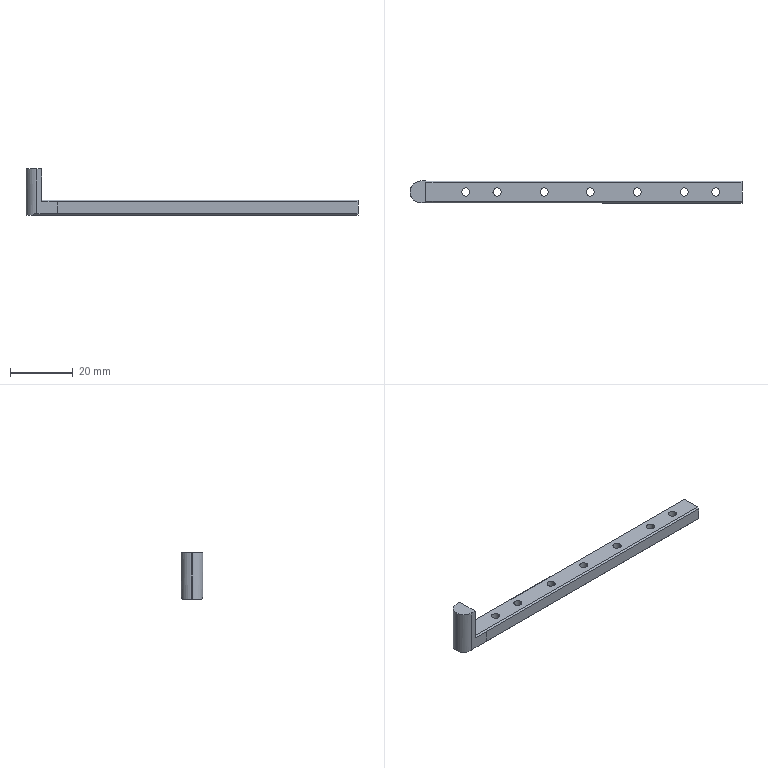Part | SolidWorks | features Chamfer 1, Extrusion 1, Fillet 1, ICE 1 | 1 solid | 34 faces | box 105.759 x 6.991 x 14.8 mm | volume 3589 mm3 | plane 18 | cylinder 16 | commonest cylinder face diameters 2.6 x14 6.98 x2
STEP:
#1=CARTESIAN_POINT('',(-94.656,-26.837,4.8));
#2=VERTEX_POINT('',#1);
#3=CARTESIAN_POINT('',(-92.056,-26.837,4.8));
#4=VERTEX_POINT('',#3);
#5=CARTESIAN_POINT('',(-93.356,-26.837,4.8));
#6=DIRECTION('',(0.,0.,1.));
#7=DIRECTION('',(1.,0.,0.));
#8=AXIS2_PLACEMENT_3D('',#5,#6,#7);
#9=CIRCLE('',#8,1.3);
#10=EDGE_CURVE('',#2,#4,#9,.T.);
#11=ORIENTED_EDGE('',*,*,#10,.T.);
#12=CARTESIAN_POINT('',(-92.056,-26.837,0.));
#13=VERTEX_POINT('',#12);
#14=CARTESIAN_POINT('',(-92.056,-26.837,4.8));
#15=DIRECTION('',(0.,0.,-1.));
#16=VECTOR('',#15,1000.);
#17=LINE('',#14,#16);
#18=EDGE_CURVE('',#4,#13,#17,.T.);
#19=ORIENTED_EDGE('',*,*,#18,.T.);
#20=CARTESIAN_POINT('',(-94.656,-26.837,0.));
#21=VERTEX_POINT('',#20);
#22=CARTESIAN_POINT('',(-93.356,-26.837,0.));
#23=DIRECTION('',(0.,0.,1.));
#24=DIRECTION('',(1.,0.,0.));
#25=AXIS2_PLACEMENT_3D('',#22,#23,#24);
#26=CIRCLE('',#25,1.3);
#27=EDGE_CURVE('',#21,#13,#26,.T.);
#28=ORIENTED_EDGE('',*,*,#27,.F.);
#29=CARTESIAN_POINT('',(-94.656,-26.837,4.8));
#30=DIRECTION('',(0.,0.,-1.));
#31=VECTOR('',#30,1000.);
#32=LINE('',#29,#31);
#33=EDGE_CURVE('',#2,#21,#32,.T.);
#34=ORIENTED_EDGE('',*,*,#33,.F.);
#35=EDGE_LOOP('',(#11,#19,#28,#34));
#36=FACE_OUTER_BOUND('',#35,.T.);
#37=CARTESIAN_POINT('',(-93.356,-26.837,4.8));
#38=DIRECTION('',(0.,0.,-1.));
#39=DIRECTION('',(-1.,0.,0.));
#40=AXIS2_PLACEMENT_3D('',#37,#38,#39);
#41=CYLINDRICAL_SURFACE('',#40,1.3);
#42=ADVANCED_FACE('',(#36),#41,.F.);
#43=CARTESIAN_POINT('',(-104.656,-26.837,4.8));
#44=VERTEX_POINT('',#43);
#45=CARTESIAN_POINT('',(-102.056,-26.837,4.8));
#46=VERTEX_POINT('',#45);
#47=CARTESIAN_POINT('',(-103.356,-26.837,4.8));
#48=DIRECTION('',(0.,0.,1.));
#49=DIRECTION('',(1.,0.,0.));
#50=AXIS2_PLACEMENT_3D('',#47,#48,#49);
#51=CIRCLE('',#50,1.3);
#52=EDGE_CURVE('',#44,#46,#51,.T.);
#53=ORIENTED_EDGE('',*,*,#52,.T.);
#54=CARTESIAN_POINT('',(-102.056,-26.837,0.));
#55=VERTEX_POINT('',#54);
#56=CARTESIAN_POINT('',(-102.056,-26.837,4.8));
#57=DIRECTION('',(0.,0.,-1.));
#58=VECTOR('',#57,1000.);
#59=LINE('',#56,#58);
#60=EDGE_CURVE('',#46,#55,#59,.T.);
#61=ORIENTED_EDGE('',*,*,#60,.T.);
#62=CARTESIAN_POINT('',(-104.656,-26.837,0.));
#63=VERTEX_POINT('',#62);
#64=CARTESIAN_POINT('',(-103.356,-26.837,0.));
#65=DIRECTION('',(0.,0.,1.));
#66=DIRECTION('',(1.,0.,0.));
#67=AXIS2_PLACEMENT_3D('',#64,#65,#66);
#68=CIRCLE('',#67,1.3);
#69=EDGE_CURVE('',#63,#55,#68,.T.);
#70=ORIENTED_EDGE('',*,*,#69,.F.);
#71=CARTESIAN_POINT('',(-104.656,-26.837,4.8));
#72=DIRECTION('',(0.,0.,-1.));
#73=VECTOR('',#72,1000.);
#74=LINE('',#71,#73);
#75=EDGE_CURVE('',#44,#63,#74,.T.);
#76=ORIENTED_EDGE('',*,*,#75,.F.);
#77=EDGE_LOOP('',(#53,#61,#70,#76));
#78=FACE_OUTER_BOUND('',#77,.T.);
#79=CARTESIAN_POINT('',(-103.356,-26.837,4.8));
#80=DIRECTION('',(0.,0.,-1.));
#81=DIRECTION('',(-1.,0.,0.));
#82=AXIS2_PLACEMENT_3D('',#79,#80,#81);
#83=CYLINDRICAL_SURFACE('',#82,1.3);
#84=ADVANCED_FACE('',(#78),#83,.F.);
#85=CARTESIAN_POINT('',(-119.656,-26.837,4.8));
#86=VERTEX_POINT('',#85);
#87=CARTESIAN_POINT('',(-117.056,-26.837,4.8));
#88=VERTEX_POINT('',#87);
#89=CARTESIAN_POINT('',(-118.356,-26.837,4.8));
#90=DIRECTION('',(0.,0.,1.));
#91=DIRECTION('',(1.,0.,0.));
#92=AXIS2_PLACEMENT_3D('',#89,#90,#91);
#93=CIRCLE('',#92,1.3);
#94=EDGE_CURVE('',#86,#88,#93,.T.);
#95=ORIENTED_EDGE('',*,*,#94,.T.);
#96=CARTESIAN_POINT('',(-117.056,-26.837,0.));
#97=VERTEX_POINT('',#96);
#98=CARTESIAN_POINT('',(-117.056,-26.837,4.8));
#99=DIRECTION('',(0.,0.,-1.));
#100=VECTOR('',#99,1000.);
#101=LINE('',#98,#100);
#102=EDGE_CURVE('',#88,#97,#101,.T.);
#103=ORIENTED_EDGE('',*,*,#102,.T.);
#104=CARTESIAN_POINT('',(-119.656,-26.837,0.));
#105=VERTEX_POINT('',#104);
#106=CARTESIAN_POINT('',(-118.356,-26.837,0.));
#107=DIRECTION('',(0.,0.,1.));
#108=DIRECTION('',(1.,0.,0.));
#109=AXIS2_PLACEMENT_3D('',#106,#107,#108);
#110=CIRCLE('',#109,1.3);
#111=EDGE_CURVE('',#105,#97,#110,.T.);
#112=ORIENTED_EDGE('',*,*,#111,.F.);
#113=CARTESIAN_POINT('',(-119.656,-26.837,4.8));
#114=DIRECTION('',(0.,0.,-1.));
#115=VECTOR('',#114,1000.);
#116=LINE('',#113,#115);
#117=EDGE_CURVE('',#86,#105,#116,.T.);
#118=ORIENTED_EDGE('',*,*,#117,.F.);
#119=EDGE_LOOP('',(#95,#103,#112,#118));
#120=FACE_OUTER_BOUND('',#119,.T.);
#121=CARTESIAN_POINT('',(-118.356,-26.837,4.8));
#122=DIRECTION('',(0.,0.,-1.));
#123=DIRECTION('',(-1.,0.,0.));
#124=AXIS2_PLACEMENT_3D('',#121,#122,#123);
#125=CYLINDRICAL_SURFACE('',#124,1.3);
#126=ADVANCED_FACE('',(#120),#125,.F.);
#127=CARTESIAN_POINT('',(-164.311,-26.837,4.8));
#128=VERTEX_POINT('',#127);
#129=CARTESIAN_POINT('',(-161.711,-26.837,4.8));
#130=VERTEX_POINT('',#129);
#131=CARTESIAN_POINT('',(-163.011,-26.837,4.8));
#132=DIRECTION('',(0.,0.,1.));
#133=DIRECTION('',(1.,0.,0.));
#134=AXIS2_PLACEMENT_3D('',#131,#132,#133);
#135=CIRCLE('',#134,1.3);
#136=EDGE_CURVE('',#128,#130,#135,.T.);
#137=ORIENTED_EDGE('',*,*,#136,.T.);
#138=CARTESIAN_POINT('',(-161.711,-26.837,0.));
#139=VERTEX_POINT('',#138);
#140=CARTESIAN_POINT('',(-161.711,-26.837,4.8));
#141=DIRECTION('',(0.,0.,-1.));
#142=VECTOR('',#141,1000.);
#143=LINE('',#140,#142);
#144=EDGE_CURVE('',#130,#139,#143,.T.);
#145=ORIENTED_EDGE('',*,*,#144,.T.);
#146=CARTESIAN_POINT('',(-164.311,-26.837,0.));
#147=VERTEX_POINT('',#146);
#148=CARTESIAN_POINT('',(-163.011,-26.837,0.));
#149=DIRECTION('',(0.,0.,1.));
#150=DIRECTION('',(1.,0.,0.));
#151=AXIS2_PLACEMENT_3D('',#148,#149,#150);
#152=CIRCLE('',#151,1.3);
#153=EDGE_CURVE('',#147,#139,#152,.T.);
#154=ORIENTED_EDGE('',*,*,#153,.F.);
#155=CARTESIAN_POINT('',(-164.311,-26.837,4.8));
#156=DIRECTION('',(0.,0.,-1.));
#157=VECTOR('',#156,1000.);
#158=LINE('',#155,#157);
#159=EDGE_CURVE('',#128,#147,#158,.T.);
#160=ORIENTED_EDGE('',*,*,#159,.F.);
#161=EDGE_LOOP('',(#137,#145,#154,#160));
#162=FACE_OUTER_BOUND('',#161,.T.);
#163=CARTESIAN_POINT('',(-163.011,-26.837,4.8));
#164=DIRECTION('',(0.,0.,-1.));
#165=DIRECTION('',(-1.,0.,0.));
#166=AXIS2_PLACEMENT_3D('',#163,#164,#165);
#167=CYLINDRICAL_SURFACE('',#166,1.3);
#168=ADVANCED_FACE('',(#162),#167,.F.);
#169=CARTESIAN_POINT('',(-149.311,-26.837,4.8));
#170=VERTEX_POINT('',#169);
#171=CARTESIAN_POINT('',(-146.711,-26.837,4.8));
#172=VERTEX_POINT('',#171);
#173=CARTESIAN_POINT('',(-148.011,-26.837,4.8));
#174=DIRECTION('',(0.,0.,1.));
#175=DIRECTION('',(1.,0.,0.));
#176=AXIS2_PLACEMENT_3D('',#173,#174,#175);
#177=CIRCLE('',#176,1.3);
#178=EDGE_CURVE('',#170,#172,#177,.T.);
#179=ORIENTED_EDGE('',*,*,#178,.T.);
#180=CARTESIAN_POINT('',(-146.711,-26.837,0.));
#181=VERTEX_POINT('',#180);
#182=CARTESIAN_POINT('',(-146.711,-26.837,4.8));
#183=DIRECTION('',(0.,0.,-1.));
#184=VECTOR('',#183,1000.);
#185=LINE('',#182,#184);
#186=EDGE_CURVE('',#172,#181,#185,.T.);
#187=ORIENTED_EDGE('',*,*,#186,.T.);
#188=CARTESIAN_POINT('',(-149.311,-26.837,0.));
#189=VERTEX_POINT('',#188);
#190=CARTESIAN_POINT('',(-148.011,-26.837,0.));
#191=DIRECTION('',(0.,0.,1.));
#192=DIRECTION('',(1.,0.,0.));
#193=AXIS2_PLACEMENT_3D('',#190,#191,#192);
#194=CIRCLE('',#193,1.3);
#195=EDGE_CURVE('',#189,#181,#194,.T.);
#196=ORIENTED_EDGE('',*,*,#195,.F.);
#197=CARTESIAN_POINT('',(-149.311,-26.837,4.8));
#198=DIRECTION('',(0.,0.,-1.));
#199=VECTOR('',#198,1000.);
#200=LINE('',#197,#199);
#201=EDGE_CURVE('',#170,#189,#200,.T.);
#202=ORIENTED_EDGE('',*,*,#201,.F.);
#203=EDGE_LOOP('',(#179,#187,#196,#202));
#204=FACE_OUTER_BOUND('',#203,.T.);
#205=CARTESIAN_POINT('',(-148.011,-26.837,4.8));
#206=DIRECTION('',(0.,0.,-1.));
#207=DIRECTION('',(-1.,0.,0.));
#208=AXIS2_PLACEMENT_3D('',#205,#206,#207);
#209=CYLINDRICAL_SURFACE('',#208,1.3);
#210=ADVANCED_FACE('',(#204),#209,.F.);
#211=CARTESIAN_POINT('',(-134.656,-26.837,4.8));
#212=VERTEX_POINT('',#211);
#213=CARTESIAN_POINT('',(-132.056,-26.837,4.8));
#214=VERTEX_POINT('',#213);
#215=CARTESIAN_POINT('',(-133.356,-26.837,4.8));
#216=DIRECTION('',(0.,0.,1.));
#217=DIRECTION('',(1.,0.,0.));
#218=AXIS2_PLACEMENT_3D('',#215,#216,#217);
#219=CIRCLE('',#218,1.3);
#220=EDGE_CURVE('',#212,#214,#219,.T.);
#221=ORIENTED_EDGE('',*,*,#220,.T.);
#222=CARTESIAN_POINT('',(-132.056,-26.837,0.));
#223=VERTEX_POINT('',#222);
#224=CARTESIAN_POINT('',(-132.056,-26.837,4.8));
#225=DIRECTION('',(0.,0.,-1.));
#226=VECTOR('',#225,1000.);
#227=LINE('',#224,#226);
#228=EDGE_CURVE('',#214,#223,#227,.T.);
#229=ORIENTED_EDGE('',*,*,#228,.T.);
#230=CARTESIAN_POINT('',(-134.656,-26.837,0.));
#231=VERTEX_POINT('',#230);
#232=CARTESIAN_POINT('',(-133.356,-26.837,0.));
#233=DIRECTION('',(0.,0.,1.));
#234=DIRECTION('',(1.,0.,0.));
#235=AXIS2_PLACEMENT_3D('',#232,#233,#234);
#236=CIRCLE('',#235,1.3);
#237=EDGE_CURVE('',#231,#223,#236,.T.);
#238=ORIENTED_EDGE('',*,*,#237,.F.);
#239=CARTESIAN_POINT('',(-134.656,-26.837,4.8));
#240=DIRECTION('',(0.,0.,-1.));
#241=VECTOR('',#240,1000.);
#242=LINE('',#239,#241);
#243=EDGE_CURVE('',#212,#231,#242,.T.);
#244=ORIENTED_EDGE('',*,*,#243,.F.);
#245=EDGE_LOOP('',(#221,#229,#238,#244));
#246=FACE_OUTER_BOUND('',#245,.T.);
#247=CARTESIAN_POINT('',(-133.356,-26.837,4.8));
#248=DIRECTION('',(0.,0.,-1.));
#249=DIRECTION('',(-1.,0.,0.));
#250=AXIS2_PLACEMENT_3D('',#247,#248,#249);
#251=CYLINDRICAL_SURFACE('',#250,1.3);
#252=ADVANCED_FACE('',(#246),#251,.F.);
#253=CARTESIAN_POINT('',(-174.311,-26.837,4.8));
#254=VERTEX_POINT('',#253);
#255=CARTESIAN_POINT('',(-171.711,-26.837,4.8));
#256=VERTEX_POINT('',#255);
#257=CARTESIAN_POINT('',(-173.011,-26.837,4.8));
#258=DIRECTION('',(0.,0.,1.));
#259=DIRECTION('',(1.,0.,0.));
#260=AXIS2_PLACEMENT_3D('',#257,#258,#259);
#261=CIRCLE('',#260,1.3);
#262=EDGE_CURVE('',#254,#256,#261,.T.);
#263=ORIENTED_EDGE('',*,*,#262,.T.);
#264=CARTESIAN_POINT('',(-171.711,-26.837,0.));
#265=VERTEX_POINT('',#264);
#266=CARTESIAN_POINT('',(-171.711,-26.837,4.8));
#267=DIRECTION('',(0.,0.,-1.));
#268=VECTOR('',#267,1000.);
#269=LINE('',#266,#268);
#270=EDGE_CURVE('',#256,#265,#269,.T.);
#271=ORIENTED_EDGE('',*,*,#270,.T.);
#272=CARTESIAN_POINT('',(-174.311,-26.837,0.));
#273=VERTEX_POINT('',#272);
#274=CARTESIAN_POINT('',(-173.011,-26.837,0.));
#275=DIRECTION('',(0.,0.,1.));
#276=DIRECTION('',(1.,0.,0.));
#277=AXIS2_PLACEMENT_3D('',#274,#275,#276);
#278=CIRCLE('',#277,1.3);
#279=EDGE_CURVE('',#273,#265,#278,.T.);
#280=ORIENTED_EDGE('',*,*,#279,.F.);
#281=CARTESIAN_POINT('',(-174.311,-26.837,4.8));
#282=DIRECTION('',(0.,0.,-1.));
#283=VECTOR('',#282,1000.);
#284=LINE('',#281,#283);
#285=EDGE_CURVE('',#254,#273,#284,.T.);
#286=ORIENTED_EDGE('',*,*,#285,.F.);
#287=EDGE_LOOP('',(#263,#271,#280,#286));
#288=FACE_OUTER_BOUND('',#287,.T.);
#289=CARTESIAN_POINT('',(-173.011,-26.837,4.8));
#290=DIRECTION('',(0.,0.,-1.));
#291=DIRECTION('',(-1.,0.,0.));
#292=AXIS2_PLACEMENT_3D('',#289,#290,#291);
#293=CYLINDRICAL_SURFACE('',#292,1.3);
#294=ADVANCED_FACE('',(#288),#293,.F.);
#295=ORIENTED_EDGE('',*,*,#10,.F.);
#296=CARTESIAN_POINT('',(-93.356,-26.837,4.8));
#297=DIRECTION('',(0.,0.,1.));
#298=DIRECTION('',(1.,0.,0.));
#299=AXIS2_PLACEMENT_3D('',#296,#297,#298);
#300=CIRCLE('',#299,1.3);
#301=EDGE_CURVE('',#4,#2,#300,.T.);
#302=ORIENTED_EDGE('',*,*,#301,.F.);
#303=EDGE_LOOP('',(#295,#302));
#304=FACE_BOUND('',#303,.T.);
#305=ORIENTED_EDGE('',*,*,#52,.F.);
#306=CARTESIAN_POINT('',(-103.356,-26.837,4.8));
#307=DIRECTION('',(0.,0.,1.));
#308=DIRECTION('',(1.,0.,0.));
#309=AXIS2_PLACEMENT_3D('',#306,#307,#308);
#310=CIRCLE('',#309,1.3);
#311=EDGE_CURVE('',#46,#44,#310,.T.);
#312=ORIENTED_EDGE('',*,*,#311,.F.);
#313=EDGE_LOOP('',(#305,#312));
#314=FACE_BOUND('',#313,.T.);
#315=ORIENTED_EDGE('',*,*,#94,.F.);
#316=CARTESIAN_POINT('',(-118.356,-26.837,4.8));
#317=DIRECTION('',(0.,0.,1.));
#318=DIRECTION('',(1.,0.,0.));
#319=AXIS2_PLACEMENT_3D('',#316,#317,#318);
#320=CIRCLE('',#319,1.3);
#321=EDGE_CURVE('',#88,#86,#320,.T.);
#322=ORIENTED_EDGE('',*,*,#321,.F.);
#323=EDGE_LOOP('',(#315,#322));
#324=FACE_BOUND('',#323,.T.);
#325=ORIENTED_EDGE('',*,*,#136,.F.);
#326=CARTESIAN_POINT('',(-163.011,-26.837,4.8));
#327=DIRECTION('',(0.,0.,1.));
#328=DIRECTION('',(1.,0.,0.));
#329=AXIS2_PLACEMENT_3D('',#326,#327,#328);
#330=CIRCLE('',#329,1.3);
#331=EDGE_CURVE('',#130,#128,#330,.T.);
#332=ORIENTED_EDGE('',*,*,#331,.F.);
#333=EDGE_LOOP('',(#325,#332));
#334=FACE_BOUND('',#333,.T.);
#335=ORIENTED_EDGE('',*,*,#178,.F.);
#336=CARTESIAN_POINT('',(-148.011,-26.837,4.8));
#337=DIRECTION('',(0.,0.,1.));
#338=DIRECTION('',(1.,0.,0.));
#339=AXIS2_PLACEMENT_3D('',#336,#337,#338);
#340=CIRCLE('',#339,1.3);
#341=EDGE_CURVE('',#172,#170,#340,.T.);
#342=ORIENTED_EDGE('',*,*,#341,.F.);
#343=EDGE_LOOP('',(#335,#342));
#344=FACE_BOUND('',#343,.T.);
#345=ORIENTED_EDGE('',*,*,#220,.F.);
#346=CARTESIAN_POINT('',(-133.356,-26.837,4.8));
#347=DIRECTION('',(0.,0.,1.));
#348=DIRECTION('',(1.,0.,0.));
#349=AXIS2_PLACEMENT_3D('',#346,#347,#348);
#350=CIRCLE('',#349,1.3);
#351=EDGE_CURVE('',#214,#212,#350,.T.);
#352=ORIENTED_EDGE('',*,*,#351,.F.);
#353=EDGE_LOOP('',(#345,#352));
#354=FACE_BOUND('',#353,.T.);
#355=ORIENTED_EDGE('',*,*,#262,.F.);
#356=CARTESIAN_POINT('',(-173.011,-26.837,4.8));
#357=DIRECTION('',(0.,0.,1.));
#358=DIRECTION('',(1.,0.,0.));
#359=AXIS2_PLACEMENT_3D('',#356,#357,#358);
#360=CIRCLE('',#359,1.3);
#361=EDGE_CURVE('',#256,#254,#360,.T.);
#362=ORIENTED_EDGE('',*,*,#361,.F.);
#363=EDGE_LOOP('',(#355,#362));
#364=FACE_BOUND('',#363,.T.);
#365=CARTESIAN_POINT('',(-185.746,-29.829,4.8));
#366=VERTEX_POINT('',#365);
#367=CARTESIAN_POINT('',(-185.746,-23.846,4.8));
#368=VERTEX_POINT('',#367);
#369=CARTESIAN_POINT('',(-185.746,-23.346,4.8));
#370=DIRECTION('',(0.,1.,0.));
#371=VECTOR('',#370,1000.);
#372=LINE('',#369,#371);
#373=EDGE_CURVE('',#366,#368,#372,.T.);
#374=ORIENTED_EDGE('',*,*,#373,.F.);
#375=CARTESIAN_POINT('',(-180.746,-29.829,4.8));
#376=VERTEX_POINT('',#375);
#377=CARTESIAN_POINT('',(0.,-29.829,4.8));
#378=DIRECTION('',(1.,0.,0.));
#379=VECTOR('',#378,1000.);
#380=LINE('',#377,#379);
#381=EDGE_CURVE('',#366,#376,#380,.T.);
#382=ORIENTED_EDGE('',*,*,#381,.T.);
#383=CARTESIAN_POINT('',(-84.986,-29.833,4.8));
#384=VERTEX_POINT('',#383);
#385=CARTESIAN_POINT('',(-0.001305,-29.836,4.8));
#386=DIRECTION('',(1.,-0.00004375,0.));
#387=VECTOR('',#386,1000.);
#388=LINE('',#385,#387);
#389=EDGE_CURVE('',#376,#384,#388,.T.);
#390=ORIENTED_EDGE('',*,*,#389,.T.);
#391=CARTESIAN_POINT('',(-84.986,-23.841,4.8));
#392=VERTEX_POINT('',#391);
#393=CARTESIAN_POINT('',(-84.986,-23.341,4.8));
#394=DIRECTION('',(0.,1.,0.));
#395=VECTOR('',#394,1000.);
#396=LINE('',#393,#395);
#397=EDGE_CURVE('',#384,#392,#396,.T.);
#398=ORIENTED_EDGE('',*,*,#397,.T.);
#399=CARTESIAN_POINT('',(-180.746,-23.846,4.8));
#400=VERTEX_POINT('',#399);
#401=CARTESIAN_POINT('',(0.001044,-23.838,4.8));
#402=DIRECTION('',(-1.,-0.00004379,0.));
#403=VECTOR('',#402,1000.);
#404=LINE('',#401,#403);
#405=EDGE_CURVE('',#392,#400,#404,.T.);
#406=ORIENTED_EDGE('',*,*,#405,.T.);
#407=CARTESIAN_POINT('',(0.,-23.846,4.8));
#408=DIRECTION('',(-1.,0.,0.));
#409=VECTOR('',#408,1000.);
#410=LINE('',#407,#409);
#411=EDGE_CURVE('',#400,#368,#410,.T.);
#412=ORIENTED_EDGE('',*,*,#411,.T.);
#413=EDGE_LOOP('',(#374,#382,#390,#398,#406,#412));
#414=FACE_OUTER_BOUND('',#413,.T.);
#415=CARTESIAN_POINT('',(0.,0.,4.8));
#416=DIRECTION('',(0.,0.,-1.));
#417=DIRECTION('',(-1.,0.,0.));
#418=AXIS2_PLACEMENT_3D('',#415,#416,#417);
#419=PLANE('',#418);
#420=ADVANCED_FACE('',(#304,#314,#324,#334,#344,#354,#364,#414),#419,.F.);
#421=ORIENTED_EDGE('',*,*,#69,.T.);
#422=CARTESIAN_POINT('',(-103.356,-26.837,0.));
#423=DIRECTION('',(0.,0.,1.));
#424=DIRECTION('',(1.,0.,0.));
#425=AXIS2_PLACEMENT_3D('',#422,#423,#424);
#426=CIRCLE('',#425,1.3);
#427=EDGE_CURVE('',#55,#63,#426,.T.);
#428=ORIENTED_EDGE('',*,*,#427,.T.);
#429=EDGE_LOOP('',(#421,#428));
#430=FACE_BOUND('',#429,.T.);
#431=ORIENTED_EDGE('',*,*,#153,.T.);
#432=CARTESIAN_POINT('',(-163.011,-26.837,0.));
#433=DIRECTION('',(0.,0.,1.));
#434=DIRECTION('',(1.,0.,0.));
#435=AXIS2_PLACEMENT_3D('',#432,#433,#434);
#436=CIRCLE('',#435,1.3);
#437=EDGE_CURVE('',#139,#147,#436,.T.);
#438=ORIENTED_EDGE('',*,*,#437,.T.);
#439=EDGE_LOOP('',(#431,#438));
#440=FACE_BOUND('',#439,.T.);
#441=ORIENTED_EDGE('',*,*,#237,.T.);
#442=CARTESIAN_POINT('',(-133.356,-26.837,0.));
#443=DIRECTION('',(0.,0.,1.));
#444=DIRECTION('',(1.,0.,0.));
#445=AXIS2_PLACEMENT_3D('',#442,#443,#444);
#446=CIRCLE('',#445,1.3);
#447=EDGE_CURVE('',#223,#231,#446,.T.);
#448=ORIENTED_EDGE('',*,*,#447,.T.);
#449=EDGE_LOOP('',(#441,#448));
#450=FACE_BOUND('',#449,.T.);
#451=CARTESIAN_POINT('',(-84.986,-29.833,0.));
#452=VERTEX_POINT('',#451);
#453=CARTESIAN_POINT('',(-180.746,-29.829,0.));
#454=VERTEX_POINT('',#453);
#455=CARTESIAN_POINT('',(-180.746,-29.829,0.));
#456=DIRECTION('',(-1.,0.00004375,0.));
#457=VECTOR('',#456,1000.);
#458=LINE('',#455,#457);
#459=EDGE_CURVE('',#452,#454,#458,.T.);
#460=ORIENTED_EDGE('',*,*,#459,.T.);
#461=CARTESIAN_POINT('',(-189.056,-29.829,0.));
#462=VERTEX_POINT('',#461);
#463=CARTESIAN_POINT('',(-187.256,-29.829,0.));
#464=DIRECTION('',(-1.,0.,0.));
#465=VECTOR('',#464,1000.);
#466=LINE('',#463,#465);
#467=EDGE_CURVE('',#454,#462,#466,.T.);
#468=ORIENTED_EDGE('',*,*,#467,.T.);
#469=CARTESIAN_POINT('',(-190.746,-26.839,0.));
#470=VERTEX_POINT('',#469);
#471=CARTESIAN_POINT('',(-187.256,-26.839,0.));
#472=DIRECTION('',(0.,0.,-1.));
#473=DIRECTION('',(-1.,0.,0.));
#474=AXIS2_PLACEMENT_3D('',#471,#472,#473);
#475=CIRCLE('',#474,3.49);
#476=EDGE_CURVE('',#462,#470,#475,.T.);
#477=ORIENTED_EDGE('',*,*,#476,.T.);
#478=CARTESIAN_POINT('',(-190.746,-26.836,0.));
#479=VERTEX_POINT('',#478);
#480=CARTESIAN_POINT('',(-190.746,-23.346,0.));
#481=DIRECTION('',(0.,-1.,0.));
#482=VECTOR('',#481,1000.);
#483=LINE('',#480,#482);
#484=EDGE_CURVE('',#479,#470,#483,.T.);
#485=ORIENTED_EDGE('',*,*,#484,.F.);
#486=CARTESIAN_POINT('',(-189.056,-23.846,0.));
#487=VERTEX_POINT('',#486);
#488=CARTESIAN_POINT('',(-187.256,-26.836,0.));
#489=DIRECTION('',(0.,0.,-1.));
#490=DIRECTION('',(-1.,0.,0.));
#491=AXIS2_PLACEMENT_3D('',#488,#489,#490);
#492=CIRCLE('',#491,3.49);
#493=EDGE_CURVE('',#479,#487,#492,.T.);
#494=ORIENTED_EDGE('',*,*,#493,.T.);
#495=CARTESIAN_POINT('',(-180.746,-23.846,0.));
#496=VERTEX_POINT('',#495);
#497=CARTESIAN_POINT('',(-180.746,-23.846,0.));
#498=DIRECTION('',(1.,0.,0.));
#499=VECTOR('',#498,1000.);
#500=LINE('',#497,#499);
#501=EDGE_CURVE('',#487,#496,#500,.T.);
#502=ORIENTED_EDGE('',*,*,#501,.T.);
#503=CARTESIAN_POINT('',(-84.986,-23.841,0.));
#504=VERTEX_POINT('',#503);
#505=CARTESIAN_POINT('',(-84.986,-23.841,0.));
#506=DIRECTION('',(1.,0.00004379,0.));
#507=VECTOR('',#506,1000.);
#508=LINE('',#505,#507);
#509=EDGE_CURVE('',#496,#504,#508,.T.);
#510=ORIENTED_EDGE('',*,*,#509,.T.);
#511=CARTESIAN_POINT('',(-84.986,-23.341,0.));
#512=DIRECTION('',(0.,1.,0.));
#513=VECTOR('',#512,1000.);
#514=LINE('',#511,#513);
#515=EDGE_CURVE('',#452,#504,#514,.T.);
#516=ORIENTED_EDGE('',*,*,#515,.F.);
#517=EDGE_LOOP('',(#460,#468,#477,#485,#494,#502,#510,#516));
#518=FACE_OUTER_BOUND('',#517,.T.);
#519=ORIENTED_EDGE('',*,*,#279,.T.);
#520=CARTESIAN_POINT('',(-173.011,-26.837,0.));
#521=DIRECTION('',(0.,0.,1.));
#522=DIRECTION('',(1.,0.,0.));
#523=AXIS2_PLACEMENT_3D('',#520,#521,#522);
#524=CIRCLE('',#523,1.3);
#525=EDGE_CURVE('',#265,#273,#524,.T.);
#526=ORIENTED_EDGE('',*,*,#525,.T.);
#527=EDGE_LOOP('',(#519,#526));
#528=FACE_BOUND('',#527,.T.);
#529=ORIENTED_EDGE('',*,*,#195,.T.);
#530=CARTESIAN_POINT('',(-148.011,-26.837,0.));
#531=DIRECTION('',(0.,0.,1.));
#532=DIRECTION('',(1.,0.,0.));
#533=AXIS2_PLACEMENT_3D('',#530,#531,#532);
#534=CIRCLE('',#533,1.3);
#535=EDGE_CURVE('',#181,#189,#534,.T.);
#536=ORIENTED_EDGE('',*,*,#535,.T.);
#537=EDGE_LOOP('',(#529,#536));
#538=FACE_BOUND('',#537,.T.);
#539=ORIENTED_EDGE('',*,*,#111,.T.);
#540=CARTESIAN_POINT('',(-118.356,-26.837,0.));
#541=DIRECTION('',(0.,0.,1.));
#542=DIRECTION('',(1.,0.,0.));
#543=AXIS2_PLACEMENT_3D('',#540,#541,#542);
#544=CIRCLE('',#543,1.3);
#545=EDGE_CURVE('',#97,#105,#544,.T.);
#546=ORIENTED_EDGE('',*,*,#545,.T.);
#547=EDGE_LOOP('',(#539,#546));
#548=FACE_BOUND('',#547,.T.);
#549=ORIENTED_EDGE('',*,*,#27,.T.);
#550=CARTESIAN_POINT('',(-93.356,-26.837,0.));
#551=DIRECTION('',(0.,0.,1.));
#552=DIRECTION('',(1.,0.,0.));
#553=AXIS2_PLACEMENT_3D('',#550,#551,#552);
#554=CIRCLE('',#553,1.3);
#555=EDGE_CURVE('',#13,#21,#554,.T.);
#556=ORIENTED_EDGE('',*,*,#555,.T.);
#557=EDGE_LOOP('',(#549,#556));
#558=FACE_BOUND('',#557,.T.);
#559=CARTESIAN_POINT('',(0.,0.,0.));
#560=DIRECTION('',(0.,0.,-1.));
#561=DIRECTION('',(-1.,0.,0.));
#562=AXIS2_PLACEMENT_3D('',#559,#560,#561);
#563=PLANE('',#562);
#564=ADVANCED_FACE('',(#430,#440,#450,#518,#528,#538,#548,#558),#563,.T.);
#565=CARTESIAN_POINT('',(-185.746,-23.346,14.8));
#566=VERTEX_POINT('',#565);
#567=CARTESIAN_POINT('',(-185.746,-23.346,4.3));
#568=VERTEX_POINT('',#567);
#569=CARTESIAN_POINT('',(-185.746,-23.346,14.8));
#570=DIRECTION('',(0.,0.,-1.));
#571=VECTOR('',#570,1000.);
#572=LINE('',#569,#571);
#573=EDGE_CURVE('',#566,#568,#572,.T.);
#574=ORIENTED_EDGE('',*,*,#573,.T.);
#575=CARTESIAN_POINT('',(-180.746,-23.346,4.3));
#576=VERTEX_POINT('',#575);
#577=CARTESIAN_POINT('',(-190.746,-23.346,4.3));
#578=DIRECTION('',(1.,0.,0.));
#579=VECTOR('',#578,1000.);
#580=LINE('',#577,#579);
#581=EDGE_CURVE('',#568,#576,#580,.T.);
#582=ORIENTED_EDGE('',*,*,#581,.T.);
#583=CARTESIAN_POINT('',(-180.746,-23.346,0.5));
#584=VERTEX_POINT('',#583);
#585=CARTESIAN_POINT('',(-180.746,-23.346,4.8));
#586=DIRECTION('',(0.,0.,-1.));
#587=VECTOR('',#586,1000.);
#588=LINE('',#585,#587);
#589=EDGE_CURVE('',#576,#584,#588,.T.);
#590=ORIENTED_EDGE('',*,*,#589,.T.);
#591=CARTESIAN_POINT('',(-187.256,-23.346,0.5));
#592=VERTEX_POINT('',#591);
#593=CARTESIAN_POINT('',(-187.256,-23.346,0.5));
#594=DIRECTION('',(-1.,0.,0.));
#595=VECTOR('',#594,1000.);
#596=LINE('',#593,#595);
#597=EDGE_CURVE('',#584,#592,#596,.T.);
#598=ORIENTED_EDGE('',*,*,#597,.T.);
#599=CARTESIAN_POINT('',(-187.256,-23.346,14.8));
#600=VERTEX_POINT('',#599);
#601=CARTESIAN_POINT('',(-187.256,-23.346,4.8));
#602=DIRECTION('',(0.,0.,1.));
#603=VECTOR('',#602,1000.);
#604=LINE('',#601,#603);
#605=EDGE_CURVE('',#592,#600,#604,.T.);
#606=ORIENTED_EDGE('',*,*,#605,.T.);
#607=CARTESIAN_POINT('',(-190.746,-23.346,14.8));
#608=DIRECTION('',(-1.,0.,0.));
#609=VECTOR('',#608,1000.);
#610=LINE('',#607,#609);
#611=EDGE_CURVE('',#566,#600,#610,.T.);
#612=ORIENTED_EDGE('',*,*,#611,.F.);
#613=EDGE_LOOP('',(#574,#582,#590,#598,#606,#612));
#614=FACE_OUTER_BOUND('',#613,.T.);
#615=CARTESIAN_POINT('',(-190.746,-23.346,4.8));
#616=DIRECTION('',(0.,-1.,0.));
#617=DIRECTION('',(0.,0.,-1.));
#618=AXIS2_PLACEMENT_3D('',#615,#616,#617);
#619=PLANE('',#618);
#620=ADVANCED_FACE('',(#614),#619,.F.);
#621=ORIENTED_EDGE('',*,*,#484,.T.);
#622=CARTESIAN_POINT('',(-190.746,-26.839,14.8));
#623=VERTEX_POINT('',#622);
#624=CARTESIAN_POINT('',(-190.746,-26.839,4.8));
#625=DIRECTION('',(0.,0.,1.));
#626=VECTOR('',#625,1000.);
#627=LINE('',#624,#626);
#628=EDGE_CURVE('',#470,#623,#627,.T.);
#629=ORIENTED_EDGE('',*,*,#628,.T.);
#630=CARTESIAN_POINT('',(-190.746,-26.836,14.8));
#631=VERTEX_POINT('',#630);
#632=CARTESIAN_POINT('',(-190.746,-23.346,14.8));
#633=DIRECTION('',(0.,-1.,0.));
#634=VECTOR('',#633,1000.);
#635=LINE('',#632,#634);
#636=EDGE_CURVE('',#631,#623,#635,.T.);
#637=ORIENTED_EDGE('',*,*,#636,.F.);
#638=CARTESIAN_POINT('',(-190.746,-26.836,4.8));
#639=DIRECTION('',(0.,0.,-1.));
#640=VECTOR('',#639,1000.);
#641=LINE('',#638,#640);
#642=EDGE_CURVE('',#631,#479,#641,.T.);
#643=ORIENTED_EDGE('',*,*,#642,.T.);
#644=EDGE_LOOP('',(#621,#629,#637,#643));
#645=FACE_OUTER_BOUND('',#644,.T.);
#646=CARTESIAN_POINT('',(-190.746,-23.346,4.8));
#647=DIRECTION('',(1.,0.,0.));
#648=DIRECTION('',(0.,0.,-1.));
#649=AXIS2_PLACEMENT_3D('',#646,#647,#648);
#650=PLANE('',#649);
#651=ADVANCED_FACE('',(#645),#650,.F.);
#652=CARTESIAN_POINT('',(-180.746,-30.329,4.3));
#653=VERTEX_POINT('',#652);
#654=CARTESIAN_POINT('',(-180.746,-30.329,0.5));
#655=VERTEX_POINT('',#654);
#656=CARTESIAN_POINT('',(-180.746,-30.329,4.8));
#657=DIRECTION('',(0.,0.,-1.));
#658=VECTOR('',#657,1000.);
#659=LINE('',#656,#658);
#660=EDGE_CURVE('',#653,#655,#659,.T.);
#661=ORIENTED_EDGE('',*,*,#660,.F.);
#662=CARTESIAN_POINT('',(-185.746,-30.329,4.3));
#663=VERTEX_POINT('',#662);
#664=CARTESIAN_POINT('',(-180.746,-30.329,4.3));
#665=DIRECTION('',(-1.,0.,0.));
#666=VECTOR('',#665,1000.);
#667=LINE('',#664,#666);
#668=EDGE_CURVE('',#653,#663,#667,.T.);
#669=ORIENTED_EDGE('',*,*,#668,.T.);
#670=CARTESIAN_POINT('',(-185.746,-30.329,14.8));
#671=VERTEX_POINT('',#670);
#672=CARTESIAN_POINT('',(-185.746,-30.329,14.8));
#673=DIRECTION('',(0.,0.,-1.));
#674=VECTOR('',#673,1000.);
#675=LINE('',#672,#674);
#676=EDGE_CURVE('',#671,#663,#675,.T.);
#677=ORIENTED_EDGE('',*,*,#676,.F.);
#678=CARTESIAN_POINT('',(-187.256,-30.329,14.8));
#679=VERTEX_POINT('',#678);
#680=CARTESIAN_POINT('',(-190.746,-30.329,14.8));
#681=DIRECTION('',(1.,0.,0.));
#682=VECTOR('',#681,1000.);
#683=LINE('',#680,#682);
#684=EDGE_CURVE('',#679,#671,#683,.T.);
#685=ORIENTED_EDGE('',*,*,#684,.F.);
#686=CARTESIAN_POINT('',(-187.256,-30.329,0.5));
#687=VERTEX_POINT('',#686);
#688=CARTESIAN_POINT('',(-187.256,-30.329,4.8));
#689=DIRECTION('',(0.,0.,-1.));
#690=VECTOR('',#689,1000.);
#691=LINE('',#688,#690);
#692=EDGE_CURVE('',#679,#687,#691,.T.);
#693=ORIENTED_EDGE('',*,*,#692,.T.);
#694=CARTESIAN_POINT('',(-180.746,-30.329,0.5));
#695=DIRECTION('',(1.,0.,0.));
#696=VECTOR('',#695,1000.);
#697=LINE('',#694,#696);
#698=EDGE_CURVE('',#687,#655,#697,.T.);
#699=ORIENTED_EDGE('',*,*,#698,.T.);
#700=EDGE_LOOP('',(#661,#669,#677,#685,#693,#699));
#701=FACE_OUTER_BOUND('',#700,.T.);
#702=CARTESIAN_POINT('',(-180.746,-30.329,4.8));
#703=DIRECTION('',(0.,1.,0.));
#704=DIRECTION('',(-1.,0.,0.));
#705=AXIS2_PLACEMENT_3D('',#702,#703,#704);
#706=PLANE('',#705);
#707=ADVANCED_FACE('',(#701),#706,.F.);
#708=ORIENTED_EDGE('',*,*,#660,.T.);
#709=CARTESIAN_POINT('',(-84.986,-30.333,0.5));
#710=VERTEX_POINT('',#709);
#711=CARTESIAN_POINT('',(-84.986,-30.333,0.5));
#712=DIRECTION('',(1.,-0.00004375,0.));
#713=VECTOR('',#712,1000.);
#714=LINE('',#711,#713);
#715=EDGE_CURVE('',#655,#710,#714,.T.);
#716=ORIENTED_EDGE('',*,*,#715,.T.);
#717=CARTESIAN_POINT('',(-84.986,-30.333,4.3));
#718=VERTEX_POINT('',#717);
#719=CARTESIAN_POINT('',(-84.986,-30.333,4.8));
#720=DIRECTION('',(0.,0.,-1.));
#721=VECTOR('',#720,1000.);
#722=LINE('',#719,#721);
#723=EDGE_CURVE('',#718,#710,#722,.T.);
#724=ORIENTED_EDGE('',*,*,#723,.F.);
#725=CARTESIAN_POINT('',(-90.621,-30.333,4.3));
#726=DIRECTION('',(-1.,0.00004375,0.));
#727=VECTOR('',#726,1000.);
#728=LINE('',#725,#727);
#729=EDGE_CURVE('',#718,#653,#728,.T.);
#730=ORIENTED_EDGE('',*,*,#729,.T.);
#731=EDGE_LOOP('',(#708,#716,#724,#730));
#732=FACE_OUTER_BOUND('',#731,.T.);
#733=CARTESIAN_POINT('',(-90.621,-30.333,4.8));
#734=DIRECTION('',(0.00004375,1.,0.));
#735=DIRECTION('',(-1.,0.00004375,0.));
#736=AXIS2_PLACEMENT_3D('',#733,#734,#735);
#737=PLANE('',#736);
#738=ADVANCED_FACE('',(#732),#737,.F.);
#739=ORIENTED_EDGE('',*,*,#723,.T.);
#740=CARTESIAN_POINT('',(-84.986,-30.333,0.4999));
#741=DIRECTION('',(0.,0.7071,-0.7071));
#742=VECTOR('',#741,1000.);
#743=LINE('',#740,#742);
#744=EDGE_CURVE('',#710,#452,#743,.T.);
#745=ORIENTED_EDGE('',*,*,#744,.T.);
#746=ORIENTED_EDGE('',*,*,#515,.T.);
#747=CARTESIAN_POINT('',(-84.986,-23.341,0.5));
#748=VERTEX_POINT('',#747);
#749=CARTESIAN_POINT('',(-84.986,-23.344,0.4979));
#750=DIRECTION('',(0.,0.7071,0.7071));
#751=VECTOR('',#750,1000.);
#752=LINE('',#749,#751);
#753=EDGE_CURVE('',#504,#748,#752,.T.);
#754=ORIENTED_EDGE('',*,*,#753,.T.);
#755=CARTESIAN_POINT('',(-84.986,-23.341,4.3));
#756=VERTEX_POINT('',#755);
#757=CARTESIAN_POINT('',(-84.986,-23.341,4.8));
#758=DIRECTION('',(0.,0.,-1.));
#759=VECTOR('',#758,1000.);
#760=LINE('',#757,#759);
#761=EDGE_CURVE('',#756,#748,#760,.T.);
#762=ORIENTED_EDGE('',*,*,#761,.F.);
#763=CARTESIAN_POINT('',(-84.986,-23.84,4.798));
#764=DIRECTION('',(0.,-0.7071,0.7071));
#765=VECTOR('',#764,1000.);
#766=LINE('',#763,#765);
#767=EDGE_CURVE('',#756,#392,#766,.T.);
#768=ORIENTED_EDGE('',*,*,#767,.T.);
#769=ORIENTED_EDGE('',*,*,#397,.F.);
#770=CARTESIAN_POINT('',(-84.986,-29.835,4.798));
#771=DIRECTION('',(0.,-0.7071,-0.7071));
#772=VECTOR('',#771,1000.);
#773=LINE('',#770,#772);
#774=EDGE_CURVE('',#384,#718,#773,.T.);
#775=ORIENTED_EDGE('',*,*,#774,.T.);
#776=EDGE_LOOP('',(#739,#745,#746,#754,#762,#768,#769,#775));
#777=FACE_OUTER_BOUND('',#776,.T.);
#778=CARTESIAN_POINT('',(-84.986,-23.341,4.8));
#779=DIRECTION('',(-1.,0.,0.));
#780=DIRECTION('',(0.,0.,1.));
#781=AXIS2_PLACEMENT_3D('',#778,#779,#780);
#782=PLANE('',#781);
#783=ADVANCED_FACE('',(#777),#782,.F.);
#784=ORIENTED_EDGE('',*,*,#761,.T.);
#785=CARTESIAN_POINT('',(-180.746,-23.346,0.5));
#786=DIRECTION('',(-1.,-0.00004379,0.));
#787=VECTOR('',#786,1000.);
#788=LINE('',#785,#787);
#789=EDGE_CURVE('',#748,#584,#788,.T.);
#790=ORIENTED_EDGE('',*,*,#789,.T.);
#791=ORIENTED_EDGE('',*,*,#589,.F.);
#792=CARTESIAN_POINT('',(-180.746,-23.346,4.3));
#793=DIRECTION('',(1.,0.00004379,0.));
#794=VECTOR('',#793,1000.);
#795=LINE('',#792,#794);
#796=EDGE_CURVE('',#576,#756,#795,.T.);
#797=ORIENTED_EDGE('',*,*,#796,.T.);
#798=EDGE_LOOP('',(#784,#790,#791,#797));
#799=FACE_OUTER_BOUND('',#798,.T.);
#800=CARTESIAN_POINT('',(-180.746,-23.346,4.8));
#801=DIRECTION('',(0.00004379,-1.,0.));
#802=DIRECTION('',(1.,0.00004379,0.));
#803=AXIS2_PLACEMENT_3D('',#800,#801,#802);
#804=PLANE('',#803);
#805=ADVANCED_FACE('',(#799),#804,.F.);
#806=ORIENTED_EDGE('',*,*,#270,.F.);
#807=ORIENTED_EDGE('',*,*,#361,.T.);
#808=ORIENTED_EDGE('',*,*,#285,.T.);
#809=ORIENTED_EDGE('',*,*,#525,.F.);
#810=EDGE_LOOP('',(#806,#807,#808,#809));
#811=FACE_OUTER_BOUND('',#810,.T.);
#812=CARTESIAN_POINT('',(-173.011,-26.837,4.8));
#813=DIRECTION('',(0.,0.,-1.));
#814=DIRECTION('',(-1.,0.,0.));
#815=AXIS2_PLACEMENT_3D('',#812,#813,#814);
#816=CYLINDRICAL_SURFACE('',#815,1.3);
#817=ADVANCED_FACE('',(#811),#816,.F.);
#818=ORIENTED_EDGE('',*,*,#228,.F.);
#819=ORIENTED_EDGE('',*,*,#351,.T.);
#820=ORIENTED_EDGE('',*,*,#243,.T.);
#821=ORIENTED_EDGE('',*,*,#447,.F.);
#822=EDGE_LOOP('',(#818,#819,#820,#821));
#823=FACE_OUTER_BOUND('',#822,.T.);
#824=CARTESIAN_POINT('',(-133.356,-26.837,4.8));
#825=DIRECTION('',(0.,0.,-1.));
#826=DIRECTION('',(-1.,0.,0.));
#827=AXIS2_PLACEMENT_3D('',#824,#825,#826);
#828=CYLINDRICAL_SURFACE('',#827,1.3);
#829=ADVANCED_FACE('',(#823),#828,.F.);
#830=ORIENTED_EDGE('',*,*,#186,.F.);
#831=ORIENTED_EDGE('',*,*,#341,.T.);
#832=ORIENTED_EDGE('',*,*,#201,.T.);
#833=ORIENTED_EDGE('',*,*,#535,.F.);
#834=EDGE_LOOP('',(#830,#831,#832,#833));
#835=FACE_OUTER_BOUND('',#834,.T.);
#836=CARTESIAN_POINT('',(-148.011,-26.837,4.8));
#837=DIRECTION('',(0.,0.,-1.));
#838=DIRECTION('',(-1.,0.,0.));
#839=AXIS2_PLACEMENT_3D('',#836,#837,#838);
#840=CYLINDRICAL_SURFACE('',#839,1.3);
#841=ADVANCED_FACE('',(#835),#840,.F.);
#842=ORIENTED_EDGE('',*,*,#144,.F.);
#843=ORIENTED_EDGE('',*,*,#331,.T.);
#844=ORIENTED_EDGE('',*,*,#159,.T.);
#845=ORIENTED_EDGE('',*,*,#437,.F.);
#846=EDGE_LOOP('',(#842,#843,#844,#845));
#847=FACE_OUTER_BOUND('',#846,.T.);
#848=CARTESIAN_POINT('',(-163.011,-26.837,4.8));
#849=DIRECTION('',(0.,0.,-1.));
#850=DIRECTION('',(-1.,0.,0.));
#851=AXIS2_PLACEMENT_3D('',#848,#849,#850);
#852=CYLINDRICAL_SURFACE('',#851,1.3);
#853=ADVANCED_FACE('',(#847),#852,.F.);
#854=ORIENTED_EDGE('',*,*,#102,.F.);
#855=ORIENTED_EDGE('',*,*,#321,.T.);
#856=ORIENTED_EDGE('',*,*,#117,.T.);
#857=ORIENTED_EDGE('',*,*,#545,.F.);
#858=EDGE_LOOP('',(#854,#855,#856,#857));
#859=FACE_OUTER_BOUND('',#858,.T.);
#860=CARTESIAN_POINT('',(-118.356,-26.837,4.8));
#861=DIRECTION('',(0.,0.,-1.));
#862=DIRECTION('',(-1.,0.,0.));
#863=AXIS2_PLACEMENT_3D('',#860,#861,#862);
#864=CYLINDRICAL_SURFACE('',#863,1.3);
#865=ADVANCED_FACE('',(#859),#864,.F.);
#866=ORIENTED_EDGE('',*,*,#60,.F.);
#867=ORIENTED_EDGE('',*,*,#311,.T.);
#868=ORIENTED_EDGE('',*,*,#75,.T.);
#869=ORIENTED_EDGE('',*,*,#427,.F.);
#870=EDGE_LOOP('',(#866,#867,#868,#869));
#871=FACE_OUTER_BOUND('',#870,.T.);
#872=CARTESIAN_POINT('',(-103.356,-26.837,4.8));
#873=DIRECTION('',(0.,0.,-1.));
#874=DIRECTION('',(-1.,0.,0.));
#875=AXIS2_PLACEMENT_3D('',#872,#873,#874);
#876=CYLINDRICAL_SURFACE('',#875,1.3);
#877=ADVANCED_FACE('',(#871),#876,.F.);
#878=ORIENTED_EDGE('',*,*,#18,.F.);
#879=ORIENTED_EDGE('',*,*,#301,.T.);
#880=ORIENTED_EDGE('',*,*,#33,.T.);
#881=ORIENTED_EDGE('',*,*,#555,.F.);
#882=EDGE_LOOP('',(#878,#879,#880,#881));
#883=FACE_OUTER_BOUND('',#882,.T.);
#884=CARTESIAN_POINT('',(-93.356,-26.837,4.8));
#885=DIRECTION('',(0.,0.,-1.));
#886=DIRECTION('',(-1.,0.,0.));
#887=AXIS2_PLACEMENT_3D('',#884,#885,#886);
#888=CYLINDRICAL_SURFACE('',#887,1.3);
#889=ADVANCED_FACE('',(#883),#888,.F.);
#890=ORIENTED_EDGE('',*,*,#676,.T.);
#891=CARTESIAN_POINT('',(-185.746,-21.587,13.041));
#892=DIRECTION('',(0.,0.7071,0.7071));
#893=VECTOR('',#892,1000.);
#894=LINE('',#891,#893);
#895=EDGE_CURVE('',#663,#366,#894,.T.);
#896=ORIENTED_EDGE('',*,*,#895,.T.);
#897=ORIENTED_EDGE('',*,*,#373,.T.);
#898=CARTESIAN_POINT('',(-185.746,-28.596,9.55));
#899=DIRECTION('',(0.,0.7071,-0.7071));
#900=VECTOR('',#899,1000.);
#901=LINE('',#898,#900);
#902=EDGE_CURVE('',#368,#568,#901,.T.);
#903=ORIENTED_EDGE('',*,*,#902,.T.);
#904=ORIENTED_EDGE('',*,*,#573,.F.);
#905=CARTESIAN_POINT('',(-185.746,-23.346,14.8));
#906=DIRECTION('',(0.,1.,0.));
#907=VECTOR('',#906,1000.);
#908=LINE('',#905,#907);
#909=EDGE_CURVE('',#671,#566,#908,.T.);
#910=ORIENTED_EDGE('',*,*,#909,.F.);
#911=EDGE_LOOP('',(#890,#896,#897,#903,#904,#910));
#912=FACE_OUTER_BOUND('',#911,.T.);
#913=CARTESIAN_POINT('',(-185.746,-23.346,14.8));
#914=DIRECTION('',(-1.,0.,0.));
#915=DIRECTION('',(0.,0.,1.));
#916=AXIS2_PLACEMENT_3D('',#913,#914,#915);
#917=PLANE('',#916);
#918=ADVANCED_FACE('',(#912),#917,.F.);
#919=ORIENTED_EDGE('',*,*,#636,.T.);
#920=CARTESIAN_POINT('',(-187.256,-26.839,14.8));
#921=DIRECTION('',(0.,0.,1.));
#922=DIRECTION('',(1.,0.,0.));
#923=AXIS2_PLACEMENT_3D('',#920,#921,#922);
#924=CIRCLE('',#923,3.49);
#925=EDGE_CURVE('',#623,#679,#924,.T.);
#926=ORIENTED_EDGE('',*,*,#925,.T.);
#927=ORIENTED_EDGE('',*,*,#684,.T.);
#928=ORIENTED_EDGE('',*,*,#909,.T.);
#929=ORIENTED_EDGE('',*,*,#611,.T.);
#930=CARTESIAN_POINT('',(-187.256,-26.836,14.8));
#931=DIRECTION('',(0.,0.,1.));
#932=DIRECTION('',(1.,0.,0.));
#933=AXIS2_PLACEMENT_3D('',#930,#931,#932);
#934=CIRCLE('',#933,3.49);
#935=EDGE_CURVE('',#600,#631,#934,.T.);
#936=ORIENTED_EDGE('',*,*,#935,.T.);
#937=EDGE_LOOP('',(#919,#926,#927,#928,#929,#936));
#938=FACE_OUTER_BOUND('',#937,.T.);
#939=CARTESIAN_POINT('',(0.,0.,14.8));
#940=DIRECTION('',(0.,0.,1.));
#941=DIRECTION('',(1.,0.,0.));
#942=AXIS2_PLACEMENT_3D('',#939,#940,#941);
#943=PLANE('',#942);
#944=ADVANCED_FACE('',(#938),#943,.T.);
#945=ORIENTED_EDGE('',*,*,#476,.F.);
#946=CARTESIAN_POINT('',(-189.056,-29.829,0.));
#947=CARTESIAN_POINT('',(-188.509,-30.158,0.3292));
#948=CARTESIAN_POINT('',(-187.894,-30.329,0.5));
#949=CARTESIAN_POINT('',(-187.256,-30.329,0.5));
#950=(BOUNDED_CURVE()B_SPLINE_CURVE(3,(#946,#947,#948,#949),.UNSPECIFIED.,.F.,.F.)B_SPLINE_CURVE_WITH_KNOTS((4,4),(2.6,3.142),.UNSPECIFIED.)CURVE()GEOMETRIC_REPRESENTATION_ITEM()RATIONAL_B_SPLINE_CURVE((1.,0.9757,0.9757,1.))REPRESENTATION_ITEM(''));
#951=EDGE_CURVE('',#462,#687,#950,.T.);
#952=ORIENTED_EDGE('',*,*,#951,.T.);
#953=ORIENTED_EDGE('',*,*,#692,.F.);
#954=ORIENTED_EDGE('',*,*,#925,.F.);
#955=ORIENTED_EDGE('',*,*,#628,.F.);
#956=EDGE_LOOP('',(#945,#952,#953,#954,#955));
#957=FACE_OUTER_BOUND('',#956,.T.);
#958=CARTESIAN_POINT('',(-187.256,-26.839,4.8));
#959=DIRECTION('',(0.,0.,-1.));
#960=DIRECTION('',(-1.,0.,0.));
#961=AXIS2_PLACEMENT_3D('',#958,#959,#960);
#962=CYLINDRICAL_SURFACE('',#961,3.49);
#963=ADVANCED_FACE('',(#957),#962,.T.);
#964=ORIENTED_EDGE('',*,*,#605,.F.);
#965=CARTESIAN_POINT('',(-187.256,-23.346,0.5));
#966=CARTESIAN_POINT('',(-187.894,-23.346,0.5));
#967=CARTESIAN_POINT('',(-188.509,-23.516,0.3292));
#968=CARTESIAN_POINT('',(-189.056,-23.846,0.));
#969=(BOUNDED_CURVE()B_SPLINE_CURVE(3,(#965,#966,#967,#968),.UNSPECIFIED.,.F.,.F.)B_SPLINE_CURVE_WITH_KNOTS((4,4),(3.142,3.683),.UNSPECIFIED.)CURVE()GEOMETRIC_REPRESENTATION_ITEM()RATIONAL_B_SPLINE_CURVE((1.,0.9757,0.9757,1.))REPRESENTATION_ITEM(''));
#970=EDGE_CURVE('',#592,#487,#969,.T.);
#971=ORIENTED_EDGE('',*,*,#970,.T.);
#972=ORIENTED_EDGE('',*,*,#493,.F.);
#973=ORIENTED_EDGE('',*,*,#642,.F.);
#974=ORIENTED_EDGE('',*,*,#935,.F.);
#975=EDGE_LOOP('',(#964,#971,#972,#973,#974));
#976=FACE_OUTER_BOUND('',#975,.T.);
#977=CARTESIAN_POINT('',(-187.256,-26.836,4.8));
#978=DIRECTION('',(0.,0.,-1.));
#979=DIRECTION('',(-1.,0.,0.));
#980=AXIS2_PLACEMENT_3D('',#977,#978,#979);
#981=CYLINDRICAL_SURFACE('',#980,3.49);
#982=ADVANCED_FACE('',(#976),#981,.T.);
#983=ORIENTED_EDGE('',*,*,#767,.F.);
#984=ORIENTED_EDGE('',*,*,#796,.F.);
#985=CARTESIAN_POINT('',(-180.746,-23.846,4.8));
#986=DIRECTION('',(-0.00003096,0.7071,-0.7071));
#987=VECTOR('',#986,1000.);
#988=LINE('',#985,#987);
#989=EDGE_CURVE('',#400,#576,#988,.T.);
#990=ORIENTED_EDGE('',*,*,#989,.F.);
#991=ORIENTED_EDGE('',*,*,#405,.F.);
#992=EDGE_LOOP('',(#983,#984,#990,#991));
#993=FACE_OUTER_BOUND('',#992,.T.);
#994=CARTESIAN_POINT('',(0.001044,-23.838,4.8));
#995=DIRECTION('',(0.00003096,-0.7071,-0.7071));
#996=DIRECTION('',(-1.,-0.00004379,0.));
#997=AXIS2_PLACEMENT_3D('',#994,#995,#996);
#998=PLANE('',#997);
#999=ADVANCED_FACE('',(#993),#998,.F.);
#1000=ORIENTED_EDGE('',*,*,#989,.T.);
#1001=ORIENTED_EDGE('',*,*,#581,.F.);
#1002=ORIENTED_EDGE('',*,*,#902,.F.);
#1003=ORIENTED_EDGE('',*,*,#411,.F.);
#1004=EDGE_LOOP('',(#1000,#1001,#1002,#1003));
#1005=FACE_OUTER_BOUND('',#1004,.T.);
#1006=CARTESIAN_POINT('',(0.,-23.846,4.8));
#1007=DIRECTION('',(0.,-0.7071,-0.7071));
#1008=DIRECTION('',(-1.,0.,0.));
#1009=AXIS2_PLACEMENT_3D('',#1006,#1007,#1008);
#1010=PLANE('',#1009);
#1011=ADVANCED_FACE('',(#1005),#1010,.F.);
#1012=ORIENTED_EDGE('',*,*,#753,.F.);
#1013=ORIENTED_EDGE('',*,*,#509,.F.);
#1014=CARTESIAN_POINT('',(-180.746,-23.346,0.5));
#1015=DIRECTION('',(0.00003096,-0.7071,-0.7071));
#1016=VECTOR('',#1015,1000.);
#1017=LINE('',#1014,#1016);
#1018=EDGE_CURVE('',#584,#496,#1017,.T.);
#1019=ORIENTED_EDGE('',*,*,#1018,.F.);
#1020=ORIENTED_EDGE('',*,*,#789,.F.);
#1021=EDGE_LOOP('',(#1012,#1013,#1019,#1020));
#1022=FACE_OUTER_BOUND('',#1021,.T.);
#1023=CARTESIAN_POINT('',(-180.746,-23.346,0.5));
#1024=DIRECTION('',(-0.00003096,0.7071,-0.7071));
#1025=DIRECTION('',(1.,0.00004379,0.));
#1026=AXIS2_PLACEMENT_3D('',#1023,#1024,#1025);
#1027=PLANE('',#1026);
#1028=ADVANCED_FACE('',(#1022),#1027,.T.);
#1029=ORIENTED_EDGE('',*,*,#1018,.T.);
#1030=ORIENTED_EDGE('',*,*,#501,.F.);
#1031=ORIENTED_EDGE('',*,*,#970,.F.);
#1032=ORIENTED_EDGE('',*,*,#597,.F.);
#1033=EDGE_LOOP('',(#1029,#1030,#1031,#1032));
#1034=FACE_OUTER_BOUND('',#1033,.T.);
#1035=CARTESIAN_POINT('',(-190.746,-23.346,0.5));
#1036=DIRECTION('',(0.,0.7071,-0.7071));
#1037=DIRECTION('',(1.,0.,0.));
#1038=AXIS2_PLACEMENT_3D('',#1035,#1036,#1037);
#1039=PLANE('',#1038);
#1040=ADVANCED_FACE('',(#1034),#1039,.T.);
#1041=ORIENTED_EDGE('',*,*,#774,.F.);
#1042=ORIENTED_EDGE('',*,*,#389,.F.);
#1043=CARTESIAN_POINT('',(-180.746,-30.329,4.3));
#1044=DIRECTION('',(0.00003094,0.7071,0.7071));
#1045=VECTOR('',#1044,1000.);
#1046=LINE('',#1043,#1045);
#1047=EDGE_CURVE('',#653,#376,#1046,.T.);
#1048=ORIENTED_EDGE('',*,*,#1047,.F.);
#1049=ORIENTED_EDGE('',*,*,#729,.F.);
#1050=EDGE_LOOP('',(#1041,#1042,#1048,#1049));
#1051=FACE_OUTER_BOUND('',#1050,.T.);
#1052=CARTESIAN_POINT('',(-0.001305,-29.836,4.8));
#1053=DIRECTION('',(0.00003094,0.7071,-0.7071));
#1054=DIRECTION('',(1.,-0.00004375,0.));
#1055=AXIS2_PLACEMENT_3D('',#1052,#1053,#1054);
#1056=PLANE('',#1055);
#1057=ADVANCED_FACE('',(#1051),#1056,.F.);
#1058=ORIENTED_EDGE('',*,*,#895,.F.);
#1059=ORIENTED_EDGE('',*,*,#668,.F.);
#1060=ORIENTED_EDGE('',*,*,#1047,.T.);
#1061=ORIENTED_EDGE('',*,*,#381,.F.);
#1062=EDGE_LOOP('',(#1058,#1059,#1060,#1061));
#1063=FACE_OUTER_BOUND('',#1062,.T.);
#1064=CARTESIAN_POINT('',(0.,-29.829,4.8));
#1065=DIRECTION('',(0.,0.7071,-0.7071));
#1066=DIRECTION('',(1.,0.,0.));
#1067=AXIS2_PLACEMENT_3D('',#1064,#1065,#1066);
#1068=PLANE('',#1067);
#1069=ADVANCED_FACE('',(#1063),#1068,.F.);
#1070=ORIENTED_EDGE('',*,*,#744,.F.);
#1071=ORIENTED_EDGE('',*,*,#715,.F.);
#1072=CARTESIAN_POINT('',(-180.746,-29.829,0.));
#1073=DIRECTION('',(-0.00003094,-0.7071,0.7071));
#1074=VECTOR('',#1073,1000.);
#1075=LINE('',#1072,#1074);
#1076=EDGE_CURVE('',#454,#655,#1075,.T.);
#1077=ORIENTED_EDGE('',*,*,#1076,.F.);
#1078=ORIENTED_EDGE('',*,*,#459,.F.);
#1079=EDGE_LOOP('',(#1070,#1071,#1077,#1078));
#1080=FACE_OUTER_BOUND('',#1079,.T.);
#1081=CARTESIAN_POINT('',(-90.621,-30.333,0.5));
#1082=DIRECTION('',(-0.00003094,-0.7071,-0.7071));
#1083=DIRECTION('',(-1.,0.00004375,0.));
#1084=AXIS2_PLACEMENT_3D('',#1081,#1082,#1083);
#1085=PLANE('',#1084);
#1086=ADVANCED_FACE('',(#1080),#1085,.T.);
#1087=ORIENTED_EDGE('',*,*,#951,.F.);
#1088=ORIENTED_EDGE('',*,*,#467,.F.);
#1089=ORIENTED_EDGE('',*,*,#1076,.T.);
#1090=ORIENTED_EDGE('',*,*,#698,.F.);
#1091=EDGE_LOOP('',(#1087,#1088,#1089,#1090));
#1092=FACE_OUTER_BOUND('',#1091,.T.);
#1093=CARTESIAN_POINT('',(-180.746,-30.329,0.5));
#1094=DIRECTION('',(0.,-0.7071,-0.7071));
#1095=DIRECTION('',(-1.,0.,0.));
#1096=AXIS2_PLACEMENT_3D('',#1093,#1094,#1095);
#1097=PLANE('',#1096);
#1098=ADVANCED_FACE('',(#1092),#1097,.T.);
#1099=CLOSED_SHELL('',(#42,#84,#126,#168,#210,#252,#294,#420,#564,#620,#651,#707,#738,#783,#805,#817,#829,#841,#853,#865,#877,#889,#918,#944,#963,#982,#999,#1011,#1028,#1040,#1057,#1069,#1086,#1098));
#1100=MANIFOLD_SOLID_BREP('',#1099);
#1101=CARTESIAN_POINT('',(0.,0.,0.));
#1102=DIRECTION('',(0.,0.,1.));
#1103=DIRECTION('',(1.,0.,0.));
#1104=AXIS2_PLACEMENT_3D('',#1101,#1102,#1103);
#1105=(LENGTH_UNIT()NAMED_UNIT(*)SI_UNIT(.MILLI.,.METRE.));
#1106=UNCERTAINTY_MEASURE_WITH_UNIT(LENGTH_MEASURE(0.00001),#1105,'','');
#1107=(NAMED_UNIT(*)PLANE_ANGLE_UNIT()SI_UNIT($,.RADIAN.));
#1108=(NAMED_UNIT(*)SI_UNIT($,.STERADIAN.)SOLID_ANGLE_UNIT());
#1109=(GEOMETRIC_REPRESENTATION_CONTEXT(3)GLOBAL_UNCERTAINTY_ASSIGNED_CONTEXT((#1106))GLOBAL_UNIT_ASSIGNED_CONTEXT((#1105,#1107,#1108))REPRESENTATION_CONTEXT('',''));
#1110=ADVANCED_BREP_SHAPE_REPRESENTATION('',(#1100,#1104),#1109);